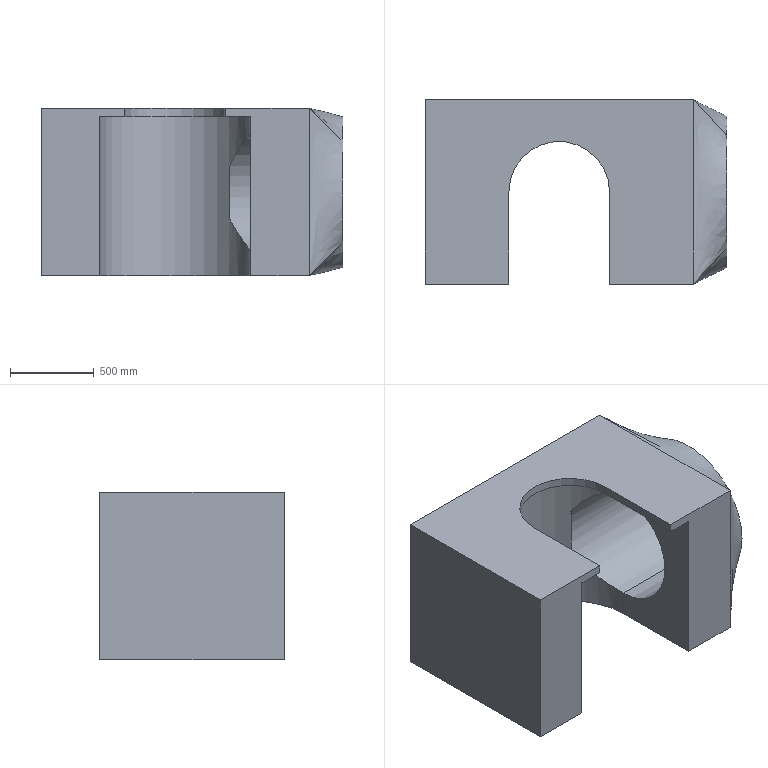Part | SolidWorks | features ICE 3, Blend 1, Extrusion 1 | 1 solid | 21 faces | box 1800 x 1100 x 1000 mm | volume 917422544 mm3 | plane 13 | cylinder 4 | spline 4 | commonest cylinder face diameters 700 x2 600 x1 900 x1
STEP:
#1=CARTESIAN_POINT('',(450.,550.,350.));
#2=VERTEX_POINT('',#1);
#3=CARTESIAN_POINT('',(450.,550.,-350.));
#4=VERTEX_POINT('',#3);
#5=CARTESIAN_POINT('',(450.,550.,0.));
#6=DIRECTION('',(1.,0.,0.));
#7=DIRECTION('',(0.,1.,0.));
#8=AXIS2_PLACEMENT_3D('',#5,#6,#7);
#9=CIRCLE('',#8,350.);
#10=EDGE_CURVE('',#2,#4,#9,.T.);
#11=ORIENTED_EDGE('',*,*,#10,.F.);
#12=CARTESIAN_POINT('',(1000.,550.,350.));
#13=VERTEX_POINT('',#12);
#14=CARTESIAN_POINT('',(324.,550.,350.));
#15=DIRECTION('',(1.,0.,0.));
#16=VECTOR('',#15,1000.);
#17=LINE('',#14,#16);
#18=EDGE_CURVE('',#2,#13,#17,.T.);
#19=ORIENTED_EDGE('',*,*,#18,.T.);
#20=CARTESIAN_POINT('',(1000.,550.,-350.));
#21=VERTEX_POINT('',#20);
#22=CARTESIAN_POINT('',(1000.,550.,0.));
#23=DIRECTION('',(1.,0.,0.));
#24=DIRECTION('',(0.,0.,-1.));
#25=AXIS2_PLACEMENT_3D('',#22,#23,#24);
#26=CIRCLE('',#25,350.);
#27=EDGE_CURVE('',#13,#21,#26,.T.);
#28=ORIENTED_EDGE('',*,*,#27,.T.);
#29=CARTESIAN_POINT('',(324.,550.,-350.));
#30=DIRECTION('',(1.,0.,0.));
#31=VECTOR('',#30,1000.);
#32=LINE('',#29,#31);
#33=EDGE_CURVE('',#4,#21,#32,.T.);
#34=ORIENTED_EDGE('',*,*,#33,.F.);
#35=EDGE_LOOP('',(#11,#19,#28,#34));
#36=FACE_OUTER_BOUND('',#35,.T.);
#37=CARTESIAN_POINT('',(324.,550.,0.));
#38=DIRECTION('',(1.,0.,0.));
#39=DIRECTION('',(0.,0.,-1.));
#40=AXIS2_PLACEMENT_3D('',#37,#38,#39);
#41=CYLINDRICAL_SURFACE('',#40,350.);
#42=ADVANCED_FACE('',(#36),#41,.F.);
#43=CARTESIAN_POINT('',(-300.,0.,500.));
#44=VERTEX_POINT('',#43);
#45=CARTESIAN_POINT('',(-300.,0.,450.));
#46=VERTEX_POINT('',#45);
#47=CARTESIAN_POINT('',(-300.,0.,500.));
#48=DIRECTION('',(0.,0.,-1.));
#49=VECTOR('',#48,1000.);
#50=LINE('',#47,#49);
#51=EDGE_CURVE('',#44,#46,#50,.T.);
#52=ORIENTED_EDGE('',*,*,#51,.F.);
#53=CARTESIAN_POINT('',(-800.,0.,500.));
#54=VERTEX_POINT('',#53);
#55=CARTESIAN_POINT('',(-800.,0.,500.));
#56=DIRECTION('',(1.,0.,0.));
#57=VECTOR('',#56,1000.);
#58=LINE('',#55,#57);
#59=EDGE_CURVE('',#54,#44,#58,.T.);
#60=ORIENTED_EDGE('',*,*,#59,.F.);
#61=CARTESIAN_POINT('',(-800.,0.,-500.));
#62=VERTEX_POINT('',#61);
#63=CARTESIAN_POINT('',(-800.,0.,500.));
#64=DIRECTION('',(0.,0.,1.));
#65=VECTOR('',#64,1000.);
#66=LINE('',#63,#65);
#67=EDGE_CURVE('',#62,#54,#66,.T.);
#68=ORIENTED_EDGE('',*,*,#67,.F.);
#69=CARTESIAN_POINT('',(-450.,0.,-500.));
#70=VERTEX_POINT('',#69);
#71=CARTESIAN_POINT('',(-800.,0.,-500.));
#72=DIRECTION('',(-1.,0.,0.));
#73=VECTOR('',#72,1000.);
#74=LINE('',#71,#73);
#75=EDGE_CURVE('',#70,#62,#74,.T.);
#76=ORIENTED_EDGE('',*,*,#75,.F.);
#77=CARTESIAN_POINT('',(-450.,0.,450.));
#78=VERTEX_POINT('',#77);
#79=CARTESIAN_POINT('',(-450.,0.,0.));
#80=DIRECTION('',(0.,0.,-1.));
#81=VECTOR('',#80,1000.);
#82=LINE('',#79,#81);
#83=EDGE_CURVE('',#78,#70,#82,.T.);
#84=ORIENTED_EDGE('',*,*,#83,.F.);
#85=CARTESIAN_POINT('',(0.,0.,450.));
#86=DIRECTION('',(1.,0.,0.));
#87=VECTOR('',#86,1000.);
#88=LINE('',#85,#87);
#89=EDGE_CURVE('',#78,#46,#88,.T.);
#90=ORIENTED_EDGE('',*,*,#89,.T.);
#91=EDGE_LOOP('',(#52,#60,#68,#76,#84,#90));
#92=FACE_OUTER_BOUND('',#91,.T.);
#93=CARTESIAN_POINT('',(0.,0.,0.));
#94=DIRECTION('',(0.,-1.,0.));
#95=DIRECTION('',(0.,0.,-1.));
#96=AXIS2_PLACEMENT_3D('',#93,#94,#95);
#97=PLANE('',#96);
#98=ADVANCED_FACE('',(#92),#97,.T.);
#99=CARTESIAN_POINT('',(-450.,550.,-500.));
#100=VERTEX_POINT('',#99);
#101=CARTESIAN_POINT('',(450.,550.,-500.));
#102=VERTEX_POINT('',#101);
#103=CARTESIAN_POINT('',(0.,550.,-500.));
#104=DIRECTION('',(0.,0.,-1.));
#105=DIRECTION('',(-1.,0.,0.));
#106=AXIS2_PLACEMENT_3D('',#103,#104,#105);
#107=CIRCLE('',#106,450.);
#108=EDGE_CURVE('',#100,#102,#107,.T.);
#109=ORIENTED_EDGE('',*,*,#108,.F.);
#110=CARTESIAN_POINT('',(-450.,550.,-500.));
#111=DIRECTION('',(0.,1.,0.));
#112=VECTOR('',#111,1000.);
#113=LINE('',#110,#112);
#114=EDGE_CURVE('',#70,#100,#113,.T.);
#115=ORIENTED_EDGE('',*,*,#114,.F.);
#116=ORIENTED_EDGE('',*,*,#75,.T.);
#117=CARTESIAN_POINT('',(-800.,1100.,-500.));
#118=VERTEX_POINT('',#117);
#119=CARTESIAN_POINT('',(-800.,1100.,-500.));
#120=DIRECTION('',(0.,-1.,0.));
#121=VECTOR('',#120,1000.);
#122=LINE('',#119,#121);
#123=EDGE_CURVE('',#118,#62,#122,.T.);
#124=ORIENTED_EDGE('',*,*,#123,.F.);
#125=CARTESIAN_POINT('',(800.,1100.,-500.));
#126=VERTEX_POINT('',#125);
#127=CARTESIAN_POINT('',(-800.,1100.,-500.));
#128=DIRECTION('',(-1.,0.,0.));
#129=VECTOR('',#128,1000.);
#130=LINE('',#127,#129);
#131=EDGE_CURVE('',#126,#118,#130,.T.);
#132=ORIENTED_EDGE('',*,*,#131,.F.);
#133=CARTESIAN_POINT('',(800.,0.,-500.));
#134=VERTEX_POINT('',#133);
#135=CARTESIAN_POINT('',(800.,1100.,-500.));
#136=DIRECTION('',(0.,-1.,0.));
#137=VECTOR('',#136,1000.);
#138=LINE('',#135,#137);
#139=EDGE_CURVE('',#126,#134,#138,.T.);
#140=ORIENTED_EDGE('',*,*,#139,.T.);
#141=CARTESIAN_POINT('',(450.,0.,-500.));
#142=VERTEX_POINT('',#141);
#143=CARTESIAN_POINT('',(-800.,0.,-500.));
#144=DIRECTION('',(-1.,0.,0.));
#145=VECTOR('',#144,1000.);
#146=LINE('',#143,#145);
#147=EDGE_CURVE('',#134,#142,#146,.T.);
#148=ORIENTED_EDGE('',*,*,#147,.T.);
#149=CARTESIAN_POINT('',(450.,550.,-500.));
#150=DIRECTION('',(0.,-1.,0.));
#151=VECTOR('',#150,1000.);
#152=LINE('',#149,#151);
#153=EDGE_CURVE('',#102,#142,#152,.T.);
#154=ORIENTED_EDGE('',*,*,#153,.F.);
#155=EDGE_LOOP('',(#109,#115,#116,#124,#132,#140,#148,#154));
#156=FACE_OUTER_BOUND('',#155,.T.);
#157=CARTESIAN_POINT('',(-800.,1100.,-500.));
#158=DIRECTION('',(0.,0.,1.));
#159=DIRECTION('',(1.,0.,0.));
#160=AXIS2_PLACEMENT_3D('',#157,#158,#159);
#161=PLANE('',#160);
#162=ADVANCED_FACE('',(#156),#161,.F.);
#163=ORIENTED_EDGE('',*,*,#67,.T.);
#164=CARTESIAN_POINT('',(-800.,1100.,500.));
#165=VERTEX_POINT('',#164);
#166=CARTESIAN_POINT('',(-800.,1100.,500.));
#167=DIRECTION('',(0.,-1.,0.));
#168=VECTOR('',#167,1000.);
#169=LINE('',#166,#168);
#170=EDGE_CURVE('',#165,#54,#169,.T.);
#171=ORIENTED_EDGE('',*,*,#170,.F.);
#172=CARTESIAN_POINT('',(-800.,1100.,500.));
#173=DIRECTION('',(0.,0.,1.));
#174=VECTOR('',#173,1000.);
#175=LINE('',#172,#174);
#176=EDGE_CURVE('',#118,#165,#175,.T.);
#177=ORIENTED_EDGE('',*,*,#176,.F.);
#178=ORIENTED_EDGE('',*,*,#123,.T.);
#179=EDGE_LOOP('',(#163,#171,#177,#178));
#180=FACE_OUTER_BOUND('',#179,.T.);
#181=CARTESIAN_POINT('',(-800.,1100.,500.));
#182=DIRECTION('',(1.,0.,0.));
#183=DIRECTION('',(0.,0.,-1.));
#184=AXIS2_PLACEMENT_3D('',#181,#182,#183);
#185=PLANE('',#184);
#186=ADVANCED_FACE('',(#180),#185,.F.);
#187=ORIENTED_EDGE('',*,*,#59,.T.);
#188=CARTESIAN_POINT('',(-300.,550.,500.));
#189=VERTEX_POINT('',#188);
#190=CARTESIAN_POINT('',(-300.,1100.,500.));
#191=DIRECTION('',(0.,1.,0.));
#192=VECTOR('',#191,1000.);
#193=LINE('',#190,#192);
#194=EDGE_CURVE('',#44,#189,#193,.T.);
#195=ORIENTED_EDGE('',*,*,#194,.T.);
#196=CARTESIAN_POINT('',(300.,550.,500.));
#197=VERTEX_POINT('',#196);
#198=CARTESIAN_POINT('',(0.,550.,500.));
#199=DIRECTION('',(0.,0.,-1.));
#200=DIRECTION('',(-1.,0.,0.));
#201=AXIS2_PLACEMENT_3D('',#198,#199,#200);
#202=CIRCLE('',#201,300.);
#203=EDGE_CURVE('',#189,#197,#202,.T.);
#204=ORIENTED_EDGE('',*,*,#203,.T.);
#205=CARTESIAN_POINT('',(300.,0.,500.));
#206=VERTEX_POINT('',#205);
#207=CARTESIAN_POINT('',(300.,1100.,500.));
#208=DIRECTION('',(0.,-1.,0.));
#209=VECTOR('',#208,1000.);
#210=LINE('',#207,#209);
#211=EDGE_CURVE('',#197,#206,#210,.T.);
#212=ORIENTED_EDGE('',*,*,#211,.T.);
#213=CARTESIAN_POINT('',(800.,0.,500.));
#214=VERTEX_POINT('',#213);
#215=CARTESIAN_POINT('',(-800.,0.,500.));
#216=DIRECTION('',(1.,0.,0.));
#217=VECTOR('',#216,1000.);
#218=LINE('',#215,#217);
#219=EDGE_CURVE('',#206,#214,#218,.T.);
#220=ORIENTED_EDGE('',*,*,#219,.T.);
#221=CARTESIAN_POINT('',(800.,1100.,500.));
#222=VERTEX_POINT('',#221);
#223=CARTESIAN_POINT('',(800.,1100.,500.));
#224=DIRECTION('',(0.,-1.,0.));
#225=VECTOR('',#224,1000.);
#226=LINE('',#223,#225);
#227=EDGE_CURVE('',#222,#214,#226,.T.);
#228=ORIENTED_EDGE('',*,*,#227,.F.);
#229=CARTESIAN_POINT('',(-800.,1100.,500.));
#230=DIRECTION('',(1.,0.,0.));
#231=VECTOR('',#230,1000.);
#232=LINE('',#229,#231);
#233=EDGE_CURVE('',#165,#222,#232,.T.);
#234=ORIENTED_EDGE('',*,*,#233,.F.);
#235=ORIENTED_EDGE('',*,*,#170,.T.);
#236=EDGE_LOOP('',(#187,#195,#204,#212,#220,#228,#234,#235));
#237=FACE_OUTER_BOUND('',#236,.T.);
#238=CARTESIAN_POINT('',(-800.,1100.,500.));
#239=DIRECTION('',(0.,0.,-1.));
#240=DIRECTION('',(-1.,0.,0.));
#241=AXIS2_PLACEMENT_3D('',#238,#239,#240);
#242=PLANE('',#241);
#243=ADVANCED_FACE('',(#237),#242,.F.);
#244=CARTESIAN_POINT('',(800.,1100.,0.));
#245=DIRECTION('',(0.,0.,-1.));
#246=VECTOR('',#245,1000.);
#247=LINE('',#244,#246);
#248=EDGE_CURVE('',#222,#126,#247,.T.);
#249=ORIENTED_EDGE('',*,*,#248,.T.);
#250=ORIENTED_EDGE('',*,*,#131,.T.);
#251=ORIENTED_EDGE('',*,*,#176,.T.);
#252=ORIENTED_EDGE('',*,*,#233,.T.);
#253=EDGE_LOOP('',(#249,#250,#251,#252));
#254=FACE_OUTER_BOUND('',#253,.T.);
#255=CARTESIAN_POINT('',(0.,1100.,0.));
#256=DIRECTION('',(0.,-1.,0.));
#257=DIRECTION('',(0.,0.,-1.));
#258=AXIS2_PLACEMENT_3D('',#255,#256,#257);
#259=PLANE('',#258);
#260=ADVANCED_FACE('',(#254),#259,.F.);
#261=CARTESIAN_POINT('',(300.,0.,450.));
#262=VERTEX_POINT('',#261);
#263=CARTESIAN_POINT('',(300.,0.,500.));
#264=DIRECTION('',(0.,0.,-1.));
#265=VECTOR('',#264,1000.);
#266=LINE('',#263,#265);
#267=EDGE_CURVE('',#206,#262,#266,.T.);
#268=ORIENTED_EDGE('',*,*,#267,.T.);
#269=CARTESIAN_POINT('',(450.,0.,450.));
#270=VERTEX_POINT('',#269);
#271=CARTESIAN_POINT('',(0.,0.,450.));
#272=DIRECTION('',(1.,0.,0.));
#273=VECTOR('',#272,1000.);
#274=LINE('',#271,#273);
#275=EDGE_CURVE('',#262,#270,#274,.T.);
#276=ORIENTED_EDGE('',*,*,#275,.T.);
#277=CARTESIAN_POINT('',(450.,0.,0.));
#278=DIRECTION('',(0.,0.,1.));
#279=VECTOR('',#278,1000.);
#280=LINE('',#277,#279);
#281=EDGE_CURVE('',#142,#270,#280,.T.);
#282=ORIENTED_EDGE('',*,*,#281,.F.);
#283=ORIENTED_EDGE('',*,*,#147,.F.);
#284=CARTESIAN_POINT('',(800.,0.,0.));
#285=DIRECTION('',(0.,0.,-1.));
#286=VECTOR('',#285,1000.);
#287=LINE('',#284,#286);
#288=EDGE_CURVE('',#214,#134,#287,.T.);
#289=ORIENTED_EDGE('',*,*,#288,.F.);
#290=ORIENTED_EDGE('',*,*,#219,.F.);
#291=EDGE_LOOP('',(#268,#276,#282,#283,#289,#290));
#292=FACE_OUTER_BOUND('',#291,.T.);
#293=CARTESIAN_POINT('',(0.,0.,0.));
#294=DIRECTION('',(0.,-1.,0.));
#295=DIRECTION('',(0.,0.,-1.));
#296=AXIS2_PLACEMENT_3D('',#293,#294,#295);
#297=PLANE('',#296);
#298=ADVANCED_FACE('',(#292),#297,.T.);
#299=CARTESIAN_POINT('',(1000.,550.,0.));
#300=DIRECTION('',(1.,0.,0.));
#301=DIRECTION('',(0.,0.,-1.));
#302=AXIS2_PLACEMENT_3D('',#299,#300,#301);
#303=CIRCLE('',#302,350.);
#304=EDGE_CURVE('',#21,#13,#303,.T.);
#305=ORIENTED_EDGE('',*,*,#304,.F.);
#306=ORIENTED_EDGE('',*,*,#27,.F.);
#307=EDGE_LOOP('',(#305,#306));
#308=FACE_BOUND('',#307,.T.);
#309=CARTESIAN_POINT('',(1000.,883.964,301.609));
#310=VERTEX_POINT('',#309);
#311=CARTESIAN_POINT('',(1000.,218.021,303.793));
#312=VERTEX_POINT('',#311);
#313=CARTESIAN_POINT('',(1000.,550.,0.));
#314=DIRECTION('',(1.,0.,0.));
#315=DIRECTION('',(0.,0.,-1.));
#316=AXIS2_PLACEMENT_3D('',#313,#314,#315);
#317=CIRCLE('',#316,450.);
#318=EDGE_CURVE('',#310,#312,#317,.T.);
#319=ORIENTED_EDGE('',*,*,#318,.T.);
#320=CARTESIAN_POINT('',(1000.,216.036,-301.609));
#321=VERTEX_POINT('',#320);
#322=CARTESIAN_POINT('',(1000.,550.,0.));
#323=DIRECTION('',(1.,0.,0.));
#324=DIRECTION('',(0.,0.,-1.));
#325=AXIS2_PLACEMENT_3D('',#322,#323,#324);
#326=CIRCLE('',#325,450.);
#327=EDGE_CURVE('',#312,#321,#326,.T.);
#328=ORIENTED_EDGE('',*,*,#327,.T.);
#329=CARTESIAN_POINT('',(1000.,881.979,-303.793));
#330=VERTEX_POINT('',#329);
#331=CARTESIAN_POINT('',(1000.,550.,0.));
#332=DIRECTION('',(1.,0.,0.));
#333=DIRECTION('',(0.,0.,-1.));
#334=AXIS2_PLACEMENT_3D('',#331,#332,#333);
#335=CIRCLE('',#334,450.);
#336=EDGE_CURVE('',#321,#330,#335,.T.);
#337=ORIENTED_EDGE('',*,*,#336,.T.);
#338=CARTESIAN_POINT('',(1000.,550.,0.));
#339=DIRECTION('',(1.,0.,0.));
#340=DIRECTION('',(0.,0.,-1.));
#341=AXIS2_PLACEMENT_3D('',#338,#339,#340);
#342=CIRCLE('',#341,450.);
#343=EDGE_CURVE('',#330,#310,#342,.T.);
#344=ORIENTED_EDGE('',*,*,#343,.T.);
#345=EDGE_LOOP('',(#319,#328,#337,#344));
#346=FACE_OUTER_BOUND('',#345,.T.);
#347=CARTESIAN_POINT('',(1000.,550.,0.));
#348=DIRECTION('',(1.,0.,0.));
#349=DIRECTION('',(0.,0.,-1.));
#350=AXIS2_PLACEMENT_3D('',#347,#348,#349);
#351=PLANE('',#350);
#352=ADVANCED_FACE('',(#308,#346),#351,.T.);
#353=ORIENTED_EDGE('',*,*,#227,.T.);
#354=CARTESIAN_POINT('',(900.,109.011,401.896));
#355=DIRECTION('',(0.5634,0.6141,-0.5527));
#356=VECTOR('',#355,1000.);
#357=LINE('',#354,#356);
#358=EDGE_CURVE('',#214,#312,#357,.T.);
#359=ORIENTED_EDGE('',*,*,#358,.T.);
#360=ORIENTED_EDGE('',*,*,#318,.F.);
#361=CARTESIAN_POINT('',(900.,991.982,400.805));
#362=DIRECTION('',(-0.5634,0.6085,0.5588));
#363=VECTOR('',#362,1000.);
#364=LINE('',#361,#363);
#365=EDGE_CURVE('',#310,#222,#364,.T.);
#366=ORIENTED_EDGE('',*,*,#365,.T.);
#367=EDGE_LOOP('',(#353,#359,#360,#366));
#368=FACE_OUTER_BOUND('',#367,.T.);
#369=CARTESIAN_POINT('',(800.,1100.,500.));
#370=CARTESIAN_POINT('',(1000.,883.964,301.609));
#371=CARTESIAN_POINT('',(800.,1077.083,500.));
#372=CARTESIAN_POINT('',(1000.,874.665,311.906));
#373=CARTESIAN_POINT('',(800.,1054.167,500.));
#374=CARTESIAN_POINT('',(1000.,864.698,321.983));
#375=CARTESIAN_POINT('',(800.,1008.333,500.));
#376=CARTESIAN_POINT('',(1000.,843.427,341.48));
#377=CARTESIAN_POINT('',(800.,985.417,500.));
#378=CARTESIAN_POINT('',(1000.,832.123,350.899));
#379=CARTESIAN_POINT('',(800.,939.583,500.));
#380=CARTESIAN_POINT('',(1000.,808.221,368.843));
#381=CARTESIAN_POINT('',(800.,916.667,500.));
#382=CARTESIAN_POINT('',(1000.,795.623,377.368));
#383=CARTESIAN_POINT('',(800.,870.833,500.));
#384=CARTESIAN_POINT('',(1000.,769.231,393.288));
#385=CARTESIAN_POINT('',(800.,847.917,500.));
#386=CARTESIAN_POINT('',(1000.,755.437,400.682));
#387=CARTESIAN_POINT('',(800.,802.083,500.));
#388=CARTESIAN_POINT('',(1000.,726.801,414.115));
#389=CARTESIAN_POINT('',(800.,779.167,500.));
#390=CARTESIAN_POINT('',(1000.,711.96,420.154));
#391=CARTESIAN_POINT('',(800.,733.333,500.));
#392=CARTESIAN_POINT('',(1000.,681.434,430.68));
#393=CARTESIAN_POINT('',(800.,710.417,500.));
#394=CARTESIAN_POINT('',(1000.,665.751,435.167));
#395=CARTESIAN_POINT('',(800.,664.583,500.));
#396=CARTESIAN_POINT('',(1000.,633.789,442.434));
#397=CARTESIAN_POINT('',(800.,641.667,500.));
#398=CARTESIAN_POINT('',(1000.,617.513,445.214));
#399=CARTESIAN_POINT('',(800.,595.833,500.));
#400=CARTESIAN_POINT('',(1000.,584.65,448.969));
#401=CARTESIAN_POINT('',(800.,572.917,500.));
#402=CARTESIAN_POINT('',(1000.,568.064,449.943));
#403=CARTESIAN_POINT('',(800.,527.083,500.));
#404=CARTESIAN_POINT('',(1000.,534.887,450.052));
#405=CARTESIAN_POINT('',(800.,504.167,500.));
#406=CARTESIAN_POINT('',(1000.,518.295,449.186));
#407=CARTESIAN_POINT('',(800.,458.333,500.));
#408=CARTESIAN_POINT('',(1000.,485.409,445.647));
#409=CARTESIAN_POINT('',(800.,435.417,500.));
#410=CARTESIAN_POINT('',(1000.,469.114,442.974));
#411=CARTESIAN_POINT('',(800.,389.583,500.));
#412=CARTESIAN_POINT('',(1000.,437.106,435.917));
#413=CARTESIAN_POINT('',(800.,366.667,500.));
#414=CARTESIAN_POINT('',(1000.,421.393,431.533));
#415=CARTESIAN_POINT('',(800.,320.833,500.));
#416=CARTESIAN_POINT('',(1000.,390.799,421.207));
#417=CARTESIAN_POINT('',(800.,297.917,500.));
#418=CARTESIAN_POINT('',(1000.,375.919,415.266));
#419=CARTESIAN_POINT('',(800.,252.083,500.));
#420=CARTESIAN_POINT('',(1000.,347.195,402.02));
#421=CARTESIAN_POINT('',(800.,229.167,500.));
#422=CARTESIAN_POINT('',(1000.,333.353,394.717));
#423=CARTESIAN_POINT('',(800.,183.333,500.));
#424=CARTESIAN_POINT('',(1000.,306.857,378.971));
#425=CARTESIAN_POINT('',(800.,160.417,500.));
#426=CARTESIAN_POINT('',(1000.,294.204,370.529));
#427=CARTESIAN_POINT('',(800.,114.583,500.));
#428=CARTESIAN_POINT('',(1000.,270.185,352.742));
#429=CARTESIAN_POINT('',(800.,91.667,500.));
#430=CARTESIAN_POINT('',(1000.,258.819,343.397));
#431=CARTESIAN_POINT('',(800.,45.833,500.));
#432=CARTESIAN_POINT('',(1000.,237.42,324.04));
#433=CARTESIAN_POINT('',(800.,22.917,500.));
#434=CARTESIAN_POINT('',(1000.,227.388,314.028));
#435=CARTESIAN_POINT('',(800.,0.,500.));
#436=CARTESIAN_POINT('',(1000.,218.021,303.793));
#437=B_SPLINE_SURFACE_WITH_KNOTS('',3,1,((#369,#370),(#371,#372),(#373,#374),(#375,#376),(#377,#378),(#379,#380),(#381,#382),(#383,#384),(#385,#386),(#387,#388),(#389,#390),(#391,#392),(#393,#394),(#395,#396),(#397,#398),(#399,#400),(#401,#402),(#403,#404),(#405,#406),(#407,#408),(#409,#410),(#411,#412),(#413,#414),(#415,#416),(#417,#418),(#419,#420),(#421,#422),(#423,#424),(#425,#426),(#427,#428),(#429,#430),(#431,#432),(#433,#434),(#435,#436)),.UNSPECIFIED.,.F.,.F.,.F.,(4,2,2,2,2,2,2,2,2,2,2,2,2,2,2,2,4),(2,2),(0.,0.0625,0.125,0.1875,0.25,0.3125,0.375,0.4375,0.5,0.5625,0.625,0.6875,0.75,0.8125,0.875,0.9375,1.),(0.,1.),.UNSPECIFIED.);
#438=ADVANCED_FACE('',(#368),#437,.T.);
#439=ORIENTED_EDGE('',*,*,#288,.T.);
#440=CARTESIAN_POINT('',(900.,108.018,-400.805));
#441=DIRECTION('',(0.5634,0.6085,0.5588));
#442=VECTOR('',#441,1000.);
#443=LINE('',#440,#442);
#444=EDGE_CURVE('',#134,#321,#443,.T.);
#445=ORIENTED_EDGE('',*,*,#444,.T.);
#446=ORIENTED_EDGE('',*,*,#327,.F.);
#447=ORIENTED_EDGE('',*,*,#358,.F.);
#448=EDGE_LOOP('',(#439,#445,#446,#447));
#449=FACE_OUTER_BOUND('',#448,.T.);
#450=CARTESIAN_POINT('',(800.,0.,500.));
#451=CARTESIAN_POINT('',(1000.,218.021,303.793));
#452=CARTESIAN_POINT('',(800.,0.,479.167));
#453=CARTESIAN_POINT('',(1000.,209.507,294.488));
#454=CARTESIAN_POINT('',(800.,0.,458.333));
#455=CARTESIAN_POINT('',(1000.,201.244,284.673));
#456=CARTESIAN_POINT('',(800.,0.,416.667));
#457=CARTESIAN_POINT('',(1000.,185.381,264.05));
#458=CARTESIAN_POINT('',(800.,0.,395.833));
#459=CARTESIAN_POINT('',(1000.,177.781,253.242));
#460=CARTESIAN_POINT('',(800.,0.,354.167));
#461=CARTESIAN_POINT('',(1000.,163.399,230.691));
#462=CARTESIAN_POINT('',(800.,0.,333.333));
#463=CARTESIAN_POINT('',(1000.,156.618,218.948));
#464=CARTESIAN_POINT('',(800.,0.,291.667));
#465=CARTESIAN_POINT('',(1000.,144.029,194.616));
#466=CARTESIAN_POINT('',(800.,0.,270.833));
#467=CARTESIAN_POINT('',(1000.,138.221,182.026));
#468=CARTESIAN_POINT('',(800.,0.,229.167));
#469=CARTESIAN_POINT('',(1000.,127.719,156.123));
#470=CARTESIAN_POINT('',(800.,0.,208.333));
#471=CARTESIAN_POINT('',(1000.,123.026,142.809));
#472=CARTESIAN_POINT('',(800.,0.,166.667));
#473=CARTESIAN_POINT('',(1000.,114.872,115.607));
#474=CARTESIAN_POINT('',(800.,0.,145.833));
#475=CARTESIAN_POINT('',(1000.,111.412,101.718));
#476=CARTESIAN_POINT('',(800.,0.,104.167));
#477=CARTESIAN_POINT('',(1000.,105.818,73.541));
#478=CARTESIAN_POINT('',(800.,0.,83.333));
#479=CARTESIAN_POINT('',(1000.,103.684,59.252));
#480=CARTESIAN_POINT('',(800.,0.,41.667));
#481=CARTESIAN_POINT('',(1000.,100.8,30.468));
#482=CARTESIAN_POINT('',(800.,0.,20.833));
#483=CARTESIAN_POINT('',(1000.,100.05,15.973));
#484=CARTESIAN_POINT('',(800.,0.,-20.833));
#485=CARTESIAN_POINT('',(1000.,99.955,-13.022));
#486=CARTESIAN_POINT('',(800.,0.,-41.667));
#487=CARTESIAN_POINT('',(1000.,100.61,-27.522));
#488=CARTESIAN_POINT('',(800.,0.,-83.333));
#489=CARTESIAN_POINT('',(1000.,103.305,-56.324));
#490=CARTESIAN_POINT('',(800.,0.,-104.167));
#491=CARTESIAN_POINT('',(1000.,105.345,-70.626));
#492=CARTESIAN_POINT('',(800.,0.,-145.833));
#493=CARTESIAN_POINT('',(1000.,110.754,-98.839));
#494=CARTESIAN_POINT('',(800.,0.,-166.667));
#495=CARTESIAN_POINT('',(1000.,114.123,-112.75));
#496=CARTESIAN_POINT('',(800.,0.,-208.333));
#497=CARTESIAN_POINT('',(1000.,122.098,-140.006));
#498=CARTESIAN_POINT('',(800.,0.,-229.167));
#499=CARTESIAN_POINT('',(1000.,126.705,-153.351));
#500=CARTESIAN_POINT('',(800.,0.,-270.833));
#501=CARTESIAN_POINT('',(1000.,137.036,-179.322));
#502=CARTESIAN_POINT('',(800.,0.,-291.667));
#503=CARTESIAN_POINT('',(1000.,142.761,-191.949));
#504=CARTESIAN_POINT('',(800.,0.,-333.333));
#505=CARTESIAN_POINT('',(1000.,155.191,-216.363));
#506=CARTESIAN_POINT('',(800.,0.,-354.167));
#507=CARTESIAN_POINT('',(1000.,161.894,-228.151));
#508=CARTESIAN_POINT('',(800.,0.,-395.833));
#509=CARTESIAN_POINT('',(1000.,176.128,-250.796));
#510=CARTESIAN_POINT('',(800.,0.,-416.667));
#511=CARTESIAN_POINT('',(1000.,183.658,-261.653));
#512=CARTESIAN_POINT('',(800.,0.,-458.333));
#513=CARTESIAN_POINT('',(1000.,199.385,-282.38));
#514=CARTESIAN_POINT('',(800.,0.,-479.167));
#515=CARTESIAN_POINT('',(1000.,207.583,-292.249));
#516=CARTESIAN_POINT('',(800.,0.,-500.));
#517=CARTESIAN_POINT('',(1000.,216.036,-301.609));
#518=B_SPLINE_SURFACE_WITH_KNOTS('',3,1,((#450,#451),(#452,#453),(#454,#455),(#456,#457),(#458,#459),(#460,#461),(#462,#463),(#464,#465),(#466,#467),(#468,#469),(#470,#471),(#472,#473),(#474,#475),(#476,#477),(#478,#479),(#480,#481),(#482,#483),(#484,#485),(#486,#487),(#488,#489),(#490,#491),(#492,#493),(#494,#495),(#496,#497),(#498,#499),(#500,#501),(#502,#503),(#504,#505),(#506,#507),(#508,#509),(#510,#511),(#512,#513),(#514,#515),(#516,#517)),.UNSPECIFIED.,.F.,.F.,.F.,(4,2,2,2,2,2,2,2,2,2,2,2,2,2,2,2,4),(2,2),(0.,0.0625,0.125,0.1875,0.25,0.3125,0.375,0.4375,0.5,0.5625,0.625,0.6875,0.75,0.8125,0.875,0.9375,1.),(0.,1.),.UNSPECIFIED.);
#519=ADVANCED_FACE('',(#449),#518,.T.);
#520=ORIENTED_EDGE('',*,*,#248,.F.);
#521=ORIENTED_EDGE('',*,*,#365,.F.);
#522=ORIENTED_EDGE('',*,*,#343,.F.);
#523=CARTESIAN_POINT('',(900.,990.989,-401.896));
#524=DIRECTION('',(0.5634,-0.6141,0.5527));
#525=VECTOR('',#524,1000.);
#526=LINE('',#523,#525);
#527=EDGE_CURVE('',#126,#330,#526,.T.);
#528=ORIENTED_EDGE('',*,*,#527,.F.);
#529=EDGE_LOOP('',(#520,#521,#522,#528));
#530=FACE_OUTER_BOUND('',#529,.T.);
#531=CARTESIAN_POINT('',(800.,1100.,-500.));
#532=CARTESIAN_POINT('',(1000.,881.979,-303.793));
#533=CARTESIAN_POINT('',(800.,1100.,-479.167));
#534=CARTESIAN_POINT('',(1000.,890.493,-294.488));
#535=CARTESIAN_POINT('',(800.,1100.,-458.333));
#536=CARTESIAN_POINT('',(1000.,898.756,-284.673));
#537=CARTESIAN_POINT('',(800.,1100.,-416.667));
#538=CARTESIAN_POINT('',(1000.,914.619,-264.05));
#539=CARTESIAN_POINT('',(800.,1100.,-395.833));
#540=CARTESIAN_POINT('',(1000.,922.219,-253.242));
#541=CARTESIAN_POINT('',(800.,1100.,-354.167));
#542=CARTESIAN_POINT('',(1000.,936.601,-230.691));
#543=CARTESIAN_POINT('',(800.,1100.,-333.333));
#544=CARTESIAN_POINT('',(1000.,943.382,-218.948));
#545=CARTESIAN_POINT('',(800.,1100.,-291.667));
#546=CARTESIAN_POINT('',(1000.,955.971,-194.616));
#547=CARTESIAN_POINT('',(800.,1100.,-270.833));
#548=CARTESIAN_POINT('',(1000.,961.779,-182.026));
#549=CARTESIAN_POINT('',(800.,1100.,-229.167));
#550=CARTESIAN_POINT('',(1000.,972.281,-156.123));
#551=CARTESIAN_POINT('',(800.,1100.,-208.333));
#552=CARTESIAN_POINT('',(1000.,976.974,-142.809));
#553=CARTESIAN_POINT('',(800.,1100.,-166.667));
#554=CARTESIAN_POINT('',(1000.,985.128,-115.607));
#555=CARTESIAN_POINT('',(800.,1100.,-145.833));
#556=CARTESIAN_POINT('',(1000.,988.588,-101.718));
#557=CARTESIAN_POINT('',(800.,1100.,-104.167));
#558=CARTESIAN_POINT('',(1000.,994.182,-73.541));
#559=CARTESIAN_POINT('',(800.,1100.,-83.333));
#560=CARTESIAN_POINT('',(1000.,996.316,-59.252));
#561=CARTESIAN_POINT('',(800.,1100.,-41.667));
#562=CARTESIAN_POINT('',(1000.,999.2,-30.468));
#563=CARTESIAN_POINT('',(800.,1100.,-20.833));
#564=CARTESIAN_POINT('',(1000.,999.95,-15.973));
#565=CARTESIAN_POINT('',(800.,1100.,20.833));
#566=CARTESIAN_POINT('',(1000.,1000.045,13.022));
#567=CARTESIAN_POINT('',(800.,1100.,41.667));
#568=CARTESIAN_POINT('',(1000.,999.39,27.522));
#569=CARTESIAN_POINT('',(800.,1100.,83.333));
#570=CARTESIAN_POINT('',(1000.,996.695,56.324));
#571=CARTESIAN_POINT('',(800.,1100.,104.167));
#572=CARTESIAN_POINT('',(1000.,994.655,70.626));
#573=CARTESIAN_POINT('',(800.,1100.,145.833));
#574=CARTESIAN_POINT('',(1000.,989.246,98.839));
#575=CARTESIAN_POINT('',(800.,1100.,166.667));
#576=CARTESIAN_POINT('',(1000.,985.877,112.75));
#577=CARTESIAN_POINT('',(800.,1100.,208.333));
#578=CARTESIAN_POINT('',(1000.,977.902,140.006));
#579=CARTESIAN_POINT('',(800.,1100.,229.167));
#580=CARTESIAN_POINT('',(1000.,973.295,153.351));
#581=CARTESIAN_POINT('',(800.,1100.,270.833));
#582=CARTESIAN_POINT('',(1000.,962.964,179.322));
#583=CARTESIAN_POINT('',(800.,1100.,291.667));
#584=CARTESIAN_POINT('',(1000.,957.239,191.949));
#585=CARTESIAN_POINT('',(800.,1100.,333.333));
#586=CARTESIAN_POINT('',(1000.,944.809,216.363));
#587=CARTESIAN_POINT('',(800.,1100.,354.167));
#588=CARTESIAN_POINT('',(1000.,938.106,228.151));
#589=CARTESIAN_POINT('',(800.,1100.,395.833));
#590=CARTESIAN_POINT('',(1000.,923.872,250.796));
#591=CARTESIAN_POINT('',(800.,1100.,416.667));
#592=CARTESIAN_POINT('',(1000.,916.342,261.653));
#593=CARTESIAN_POINT('',(800.,1100.,458.333));
#594=CARTESIAN_POINT('',(1000.,900.615,282.38));
#595=CARTESIAN_POINT('',(800.,1100.,479.167));
#596=CARTESIAN_POINT('',(1000.,892.417,292.249));
#597=CARTESIAN_POINT('',(800.,1100.,500.));
#598=CARTESIAN_POINT('',(1000.,883.964,301.609));
#599=B_SPLINE_SURFACE_WITH_KNOTS('',3,1,((#531,#532),(#533,#534),(#535,#536),(#537,#538),(#539,#540),(#541,#542),(#543,#544),(#545,#546),(#547,#548),(#549,#550),(#551,#552),(#553,#554),(#555,#556),(#557,#558),(#559,#560),(#561,#562),(#563,#564),(#565,#566),(#567,#568),(#569,#570),(#571,#572),(#573,#574),(#575,#576),(#577,#578),(#579,#580),(#581,#582),(#583,#584),(#585,#586),(#587,#588),(#589,#590),(#591,#592),(#593,#594),(#595,#596),(#597,#598)),.UNSPECIFIED.,.F.,.F.,.F.,(4,2,2,2,2,2,2,2,2,2,2,2,2,2,2,2,4),(2,2),(0.,0.0625,0.125,0.1875,0.25,0.3125,0.375,0.4375,0.5,0.5625,0.625,0.6875,0.75,0.8125,0.875,0.9375,1.),(0.,1.),.UNSPECIFIED.);
#600=ADVANCED_FACE('',(#530),#599,.T.);
#601=ORIENTED_EDGE('',*,*,#139,.F.);
#602=ORIENTED_EDGE('',*,*,#527,.T.);
#603=ORIENTED_EDGE('',*,*,#336,.F.);
#604=ORIENTED_EDGE('',*,*,#444,.F.);
#605=EDGE_LOOP('',(#601,#602,#603,#604));
#606=FACE_OUTER_BOUND('',#605,.T.);
#607=CARTESIAN_POINT('',(800.,0.,-500.));
#608=CARTESIAN_POINT('',(1000.,216.036,-301.609));
#609=CARTESIAN_POINT('',(800.,22.917,-500.));
#610=CARTESIAN_POINT('',(1000.,225.335,-311.906));
#611=CARTESIAN_POINT('',(800.,45.833,-500.));
#612=CARTESIAN_POINT('',(1000.,235.302,-321.983));
#613=CARTESIAN_POINT('',(800.,91.667,-500.));
#614=CARTESIAN_POINT('',(1000.,256.573,-341.48));
#615=CARTESIAN_POINT('',(800.,114.583,-500.));
#616=CARTESIAN_POINT('',(1000.,267.877,-350.899));
#617=CARTESIAN_POINT('',(800.,160.417,-500.));
#618=CARTESIAN_POINT('',(1000.,291.779,-368.843));
#619=CARTESIAN_POINT('',(800.,183.333,-500.));
#620=CARTESIAN_POINT('',(1000.,304.377,-377.368));
#621=CARTESIAN_POINT('',(800.,229.167,-500.));
#622=CARTESIAN_POINT('',(1000.,330.769,-393.288));
#623=CARTESIAN_POINT('',(800.,252.083,-500.));
#624=CARTESIAN_POINT('',(1000.,344.563,-400.682));
#625=CARTESIAN_POINT('',(800.,297.917,-500.));
#626=CARTESIAN_POINT('',(1000.,373.199,-414.115));
#627=CARTESIAN_POINT('',(800.,320.833,-500.));
#628=CARTESIAN_POINT('',(1000.,388.04,-420.154));
#629=CARTESIAN_POINT('',(800.,366.667,-500.));
#630=CARTESIAN_POINT('',(1000.,418.566,-430.68));
#631=CARTESIAN_POINT('',(800.,389.583,-500.));
#632=CARTESIAN_POINT('',(1000.,434.249,-435.167));
#633=CARTESIAN_POINT('',(800.,435.417,-500.));
#634=CARTESIAN_POINT('',(1000.,466.211,-442.434));
#635=CARTESIAN_POINT('',(800.,458.333,-500.));
#636=CARTESIAN_POINT('',(1000.,482.487,-445.214));
#637=CARTESIAN_POINT('',(800.,504.167,-500.));
#638=CARTESIAN_POINT('',(1000.,515.35,-448.969));
#639=CARTESIAN_POINT('',(800.,527.083,-500.));
#640=CARTESIAN_POINT('',(1000.,531.936,-449.943));
#641=CARTESIAN_POINT('',(800.,572.917,-500.));
#642=CARTESIAN_POINT('',(1000.,565.113,-450.052));
#643=CARTESIAN_POINT('',(800.,595.833,-500.));
#644=CARTESIAN_POINT('',(1000.,581.705,-449.186));
#645=CARTESIAN_POINT('',(800.,641.667,-500.));
#646=CARTESIAN_POINT('',(1000.,614.591,-445.647));
#647=CARTESIAN_POINT('',(800.,664.583,-500.));
#648=CARTESIAN_POINT('',(1000.,630.886,-442.974));
#649=CARTESIAN_POINT('',(800.,710.417,-500.));
#650=CARTESIAN_POINT('',(1000.,662.894,-435.917));
#651=CARTESIAN_POINT('',(800.,733.333,-500.));
#652=CARTESIAN_POINT('',(1000.,678.607,-431.533));
#653=CARTESIAN_POINT('',(800.,779.167,-500.));
#654=CARTESIAN_POINT('',(1000.,709.201,-421.207));
#655=CARTESIAN_POINT('',(800.,802.083,-500.));
#656=CARTESIAN_POINT('',(1000.,724.081,-415.266));
#657=CARTESIAN_POINT('',(800.,847.917,-500.));
#658=CARTESIAN_POINT('',(1000.,752.805,-402.02));
#659=CARTESIAN_POINT('',(800.,870.833,-500.));
#660=CARTESIAN_POINT('',(1000.,766.647,-394.717));
#661=CARTESIAN_POINT('',(800.,916.667,-500.));
#662=CARTESIAN_POINT('',(1000.,793.143,-378.971));
#663=CARTESIAN_POINT('',(800.,939.583,-500.));
#664=CARTESIAN_POINT('',(1000.,805.796,-370.529));
#665=CARTESIAN_POINT('',(800.,985.417,-500.));
#666=CARTESIAN_POINT('',(1000.,829.815,-352.742));
#667=CARTESIAN_POINT('',(800.,1008.333,-500.));
#668=CARTESIAN_POINT('',(1000.,841.181,-343.397));
#669=CARTESIAN_POINT('',(800.,1054.167,-500.));
#670=CARTESIAN_POINT('',(1000.,862.58,-324.04));
#671=CARTESIAN_POINT('',(800.,1077.083,-500.));
#672=CARTESIAN_POINT('',(1000.,872.612,-314.028));
#673=CARTESIAN_POINT('',(800.,1100.,-500.));
#674=CARTESIAN_POINT('',(1000.,881.979,-303.793));
#675=B_SPLINE_SURFACE_WITH_KNOTS('',3,1,((#607,#608),(#609,#610),(#611,#612),(#613,#614),(#615,#616),(#617,#618),(#619,#620),(#621,#622),(#623,#624),(#625,#626),(#627,#628),(#629,#630),(#631,#632),(#633,#634),(#635,#636),(#637,#638),(#639,#640),(#641,#642),(#643,#644),(#645,#646),(#647,#648),(#649,#650),(#651,#652),(#653,#654),(#655,#656),(#657,#658),(#659,#660),(#661,#662),(#663,#664),(#665,#666),(#667,#668),(#669,#670),(#671,#672),(#673,#674)),.UNSPECIFIED.,.F.,.F.,.F.,(4,2,2,2,2,2,2,2,2,2,2,2,2,2,2,2,4),(2,2),(0.,0.0625,0.125,0.1875,0.25,0.3125,0.375,0.4375,0.5,0.5625,0.625,0.6875,0.75,0.8125,0.875,0.9375,1.),(0.,1.),.UNSPECIFIED.);
#676=ADVANCED_FACE('',(#606),#675,.T.);
#677=CARTESIAN_POINT('',(450.,550.,450.));
#678=DIRECTION('',(0.,0.,-1.));
#679=VECTOR('',#678,1000.);
#680=LINE('',#677,#679);
#681=EDGE_CURVE('',#4,#102,#680,.T.);
#682=ORIENTED_EDGE('',*,*,#681,.F.);
#683=CARTESIAN_POINT('',(324.,862.288,-158.038));
#684=VERTEX_POINT('',#683);
#685=CARTESIAN_POINT('',(450.,550.,-350.));
#686=CARTESIAN_POINT('',(450.,558.615,-350.));
#687=CARTESIAN_POINT('',(449.753,567.156,-349.682));
#688=CARTESIAN_POINT('',(448.787,584.096,-348.439));
#689=CARTESIAN_POINT('',(448.067,592.496,-347.513));
#690=CARTESIAN_POINT('',(446.173,609.158,-345.067));
#691=CARTESIAN_POINT('',(444.998,617.42,-343.548));
#692=CARTESIAN_POINT('',(442.903,629.713,-340.828));
#693=CARTESIAN_POINT('',(442.149,633.793,-339.848));
#694=CARTESIAN_POINT('',(440.531,641.92,-337.74));
#695=CARTESIAN_POINT('',(439.667,645.969,-336.612));
#696=CARTESIAN_POINT('',(436.913,658.053,-333.009));
#697=CARTESIAN_POINT('',(434.886,665.926,-330.347));
#698=CARTESIAN_POINT('',(430.484,681.33,-324.531));
#699=CARTESIAN_POINT('',(428.11,688.862,-321.377));
#700=CARTESIAN_POINT('',(423.044,703.604,-314.597));
#701=CARTESIAN_POINT('',(420.353,710.814,-310.972));
#702=CARTESIAN_POINT('',(416.097,721.398,-305.186));
#703=CARTESIAN_POINT('',(414.643,724.888,-303.2));
#704=CARTESIAN_POINT('',(412.408,730.065,-300.134));
#705=CARTESIAN_POINT('',(411.654,731.781,-299.098));
#706=CARTESIAN_POINT('',(410.13,735.194,-296.997));
#707=CARTESIAN_POINT('',(409.359,736.893,-295.931));
#708=CARTESIAN_POINT('',(405.468,745.322,-290.54));
#709=CARTESIAN_POINT('',(402.255,751.846,-286.042));
#710=CARTESIAN_POINT('',(395.658,764.489,-276.688));
#711=CARTESIAN_POINT('',(392.275,770.608,-271.832));
#712=CARTESIAN_POINT('',(385.369,782.461,-261.768));
#713=CARTESIAN_POINT('',(381.846,788.195,-256.56));
#714=CARTESIAN_POINT('',(374.693,799.296,-245.787));
#715=CARTESIAN_POINT('',(371.063,804.662,-240.223));
#716=CARTESIAN_POINT('',(365.56,812.442,-231.601));
#717=CARTESIAN_POINT('',(363.715,814.993,-228.678));
#718=CARTESIAN_POINT('',(360.026,819.983,-222.765));
#719=CARTESIAN_POINT('',(358.182,822.424,-219.773));
#720=CARTESIAN_POINT('',(352.655,829.591,-210.686));
#721=CARTESIAN_POINT('',(348.978,834.159,-204.482));
#722=CARTESIAN_POINT('',(341.684,842.89,-191.768));
#723=CARTESIAN_POINT('',(338.066,847.052,-185.258));
#724=CARTESIAN_POINT('',(330.938,854.973,-171.906));
#725=CARTESIAN_POINT('',(327.427,858.733,-165.064));
#726=CARTESIAN_POINT('',(324.,862.288,-158.038));
#727=B_SPLINE_CURVE_WITH_KNOTS('',3,(#685,#686,#687,#688,#689,#690,#691,#692,#693,#694,#695,#696,#697,#698,#699,#700,#701,#702,#703,#704,#705,#706,#707,#708,#709,#710,#711,#712,#713,#714,#715,#716,#717,#718,#719,#720,#721,#722,#723,#724,#725,#726),.UNSPECIFIED.,.F.,.F.,(4,2,2,2,2,2,2,2,2,2,2,2,2,2,2,2,2,2,2,2,4),(0.,0.02542,0.05084,0.07626,0.08897,0.1017,0.1271,0.1525,0.1779,0.1907,0.197,0.2034,0.2288,0.2542,0.2796,0.305,0.3178,0.3305,0.3559,0.3813,0.4067),.UNSPECIFIED.);
#728=EDGE_CURVE('',#4,#684,#727,.T.);
#729=ORIENTED_EDGE('',*,*,#728,.T.);
#730=CARTESIAN_POINT('',(324.,862.288,158.038));
#731=VERTEX_POINT('',#730);
#732=CARTESIAN_POINT('',(324.,862.288,450.));
#733=DIRECTION('',(0.,0.,-1.));
#734=VECTOR('',#733,1000.);
#735=LINE('',#732,#734);
#736=EDGE_CURVE('',#731,#684,#735,.T.);
#737=ORIENTED_EDGE('',*,*,#736,.F.);
#738=CARTESIAN_POINT('',(324.,862.288,158.038));
#739=CARTESIAN_POINT('',(327.434,858.725,165.079));
#740=CARTESIAN_POINT('',(330.946,854.964,171.922));
#741=CARTESIAN_POINT('',(338.066,847.052,185.257));
#742=CARTESIAN_POINT('',(341.673,842.902,191.748));
#743=CARTESIAN_POINT('',(348.934,834.213,204.407));
#744=CARTESIAN_POINT('',(352.589,829.673,210.574));
#745=CARTESIAN_POINT('',(359.902,820.197,222.603));
#746=CARTESIAN_POINT('',(363.561,815.26,228.465));
#747=CARTESIAN_POINT('',(370.849,804.973,239.892));
#748=CARTESIAN_POINT('',(374.477,799.622,245.457));
#749=CARTESIAN_POINT('',(379.869,791.268,253.584));
#750=CARTESIAN_POINT('',(381.659,788.429,256.256));
#751=CARTESIAN_POINT('',(385.217,782.636,261.526));
#752=CARTESIAN_POINT('',(386.976,779.699,264.11));
#753=CARTESIAN_POINT('',(392.187,770.764,271.706));
#754=CARTESIAN_POINT('',(395.573,764.644,276.567));
#755=CARTESIAN_POINT('',(402.143,752.069,285.884));
#756=CARTESIAN_POINT('',(405.326,745.613,290.34));
#757=CARTESIAN_POINT('',(411.462,732.352,298.847));
#758=CARTESIAN_POINT('',(414.415,725.547,302.897));
#759=CARTESIAN_POINT('',(420.062,711.568,310.579));
#760=CARTESIAN_POINT('',(422.757,704.394,314.211));
#761=CARTESIAN_POINT('',(427.854,689.65,321.036));
#762=CARTESIAN_POINT('',(430.256,682.08,324.229));
#763=CARTESIAN_POINT('',(433.054,672.347,327.926));
#764=CARTESIAN_POINT('',(433.602,670.389,328.65));
#765=CARTESIAN_POINT('',(434.672,666.464,330.061));
#766=CARTESIAN_POINT('',(435.195,664.496,330.749));
#767=CARTESIAN_POINT('',(436.725,658.573,332.76));
#768=CARTESIAN_POINT('',(437.694,654.599,334.031));
#769=CARTESIAN_POINT('',(440.445,642.604,337.63));
#770=CARTESIAN_POINT('',(442.072,634.508,339.748));
#771=CARTESIAN_POINT('',(444.893,618.111,343.412));
#772=CARTESIAN_POINT('',(446.088,609.81,344.956));
#773=CARTESIAN_POINT('',(447.538,597.2,346.829));
#774=CARTESIAN_POINT('',(447.964,592.97,347.379));
#775=CARTESIAN_POINT('',(448.516,586.583,348.089));
#776=CARTESIAN_POINT('',(448.685,584.448,348.307));
#777=CARTESIAN_POINT('',(448.993,580.163,348.704));
#778=CARTESIAN_POINT('',(449.132,578.013,348.884));
#779=CARTESIAN_POINT('',(449.751,567.264,349.68));
#780=CARTESIAN_POINT('',(450.,558.643,350.));
#781=CARTESIAN_POINT('',(450.,550.,350.));
#782=B_SPLINE_CURVE_WITH_KNOTS('',3,(#738,#739,#740,#741,#742,#743,#744,#745,#746,#747,#748,#749,#750,#751,#752,#753,#754,#755,#756,#757,#758,#759,#760,#761,#762,#763,#764,#765,#766,#767,#768,#769,#770,#771,#772,#773,#774,#775,#776,#777,#778,#779,#780,#781),.UNSPECIFIED.,.F.,.F.,(4,2,2,2,2,2,2,2,2,2,2,2,2,2,2,2,2,2,2,2,2,4),(0.,0.02545,0.0509,0.07636,0.1018,0.1273,0.14,0.1527,0.1782,0.2036,0.2291,0.2545,0.28,0.2863,0.2927,0.3054,0.3309,0.3563,0.369,0.3754,0.3818,0.4072),.UNSPECIFIED.);
#783=EDGE_CURVE('',#731,#2,#782,.T.);
#784=ORIENTED_EDGE('',*,*,#783,.T.);
#785=CARTESIAN_POINT('',(450.,550.,450.));
#786=VERTEX_POINT('',#785);
#787=CARTESIAN_POINT('',(450.,550.,450.));
#788=DIRECTION('',(0.,0.,-1.));
#789=VECTOR('',#788,1000.);
#790=LINE('',#787,#789);
#791=EDGE_CURVE('',#786,#2,#790,.T.);
#792=ORIENTED_EDGE('',*,*,#791,.F.);
#793=CARTESIAN_POINT('',(-450.,550.,450.));
#794=VERTEX_POINT('',#793);
#795=CARTESIAN_POINT('',(0.,550.,450.));
#796=DIRECTION('',(0.,0.,-1.));
#797=DIRECTION('',(-1.,0.,0.));
#798=AXIS2_PLACEMENT_3D('',#795,#796,#797);
#799=CIRCLE('',#798,450.);
#800=EDGE_CURVE('',#794,#786,#799,.T.);
#801=ORIENTED_EDGE('',*,*,#800,.F.);
#802=CARTESIAN_POINT('',(-450.,550.,450.));
#803=DIRECTION('',(0.,0.,-1.));
#804=VECTOR('',#803,1000.);
#805=LINE('',#802,#804);
#806=EDGE_CURVE('',#794,#100,#805,.T.);
#807=ORIENTED_EDGE('',*,*,#806,.T.);
#808=ORIENTED_EDGE('',*,*,#108,.T.);
#809=EDGE_LOOP('',(#682,#729,#737,#784,#792,#801,#807,#808));
#810=FACE_OUTER_BOUND('',#809,.T.);
#811=CARTESIAN_POINT('',(0.,550.,450.));
#812=DIRECTION('',(0.,0.,-1.));
#813=DIRECTION('',(-1.,0.,0.));
#814=AXIS2_PLACEMENT_3D('',#811,#812,#813);
#815=CYLINDRICAL_SURFACE('',#814,450.);
#816=ADVANCED_FACE('',(#810),#815,.F.);
#817=ORIENTED_EDGE('',*,*,#83,.T.);
#818=ORIENTED_EDGE('',*,*,#114,.T.);
#819=ORIENTED_EDGE('',*,*,#806,.F.);
#820=CARTESIAN_POINT('',(-450.,550.,450.));
#821=DIRECTION('',(0.,1.,0.));
#822=VECTOR('',#821,1000.);
#823=LINE('',#820,#822);
#824=EDGE_CURVE('',#78,#794,#823,.T.);
#825=ORIENTED_EDGE('',*,*,#824,.F.);
#826=EDGE_LOOP('',(#817,#818,#819,#825));
#827=FACE_OUTER_BOUND('',#826,.T.);
#828=CARTESIAN_POINT('',(-450.,550.,450.));
#829=DIRECTION('',(-1.,0.,0.));
#830=DIRECTION('',(0.,0.,1.));
#831=AXIS2_PLACEMENT_3D('',#828,#829,#830);
#832=PLANE('',#831);
#833=ADVANCED_FACE('',(#827),#832,.F.);
#834=ORIENTED_EDGE('',*,*,#791,.T.);
#835=ORIENTED_EDGE('',*,*,#10,.T.);
#836=ORIENTED_EDGE('',*,*,#681,.T.);
#837=ORIENTED_EDGE('',*,*,#153,.T.);
#838=ORIENTED_EDGE('',*,*,#281,.T.);
#839=CARTESIAN_POINT('',(450.,550.,450.));
#840=DIRECTION('',(0.,-1.,0.));
#841=VECTOR('',#840,1000.);
#842=LINE('',#839,#841);
#843=EDGE_CURVE('',#786,#270,#842,.T.);
#844=ORIENTED_EDGE('',*,*,#843,.F.);
#845=EDGE_LOOP('',(#834,#835,#836,#837,#838,#844));
#846=FACE_OUTER_BOUND('',#845,.T.);
#847=CARTESIAN_POINT('',(450.,550.,450.));
#848=DIRECTION('',(1.,0.,0.));
#849=DIRECTION('',(0.,1.,0.));
#850=AXIS2_PLACEMENT_3D('',#847,#848,#849);
#851=PLANE('',#850);
#852=ADVANCED_FACE('',(#846),#851,.F.);
#853=CARTESIAN_POINT('',(-300.,550.,450.));
#854=VERTEX_POINT('',#853);
#855=CARTESIAN_POINT('',(-300.,550.,450.));
#856=DIRECTION('',(0.,1.,0.));
#857=VECTOR('',#856,1000.);
#858=LINE('',#855,#857);
#859=EDGE_CURVE('',#46,#854,#858,.T.);
#860=ORIENTED_EDGE('',*,*,#859,.F.);
#861=ORIENTED_EDGE('',*,*,#89,.F.);
#862=ORIENTED_EDGE('',*,*,#824,.T.);
#863=ORIENTED_EDGE('',*,*,#800,.T.);
#864=ORIENTED_EDGE('',*,*,#843,.T.);
#865=ORIENTED_EDGE('',*,*,#275,.F.);
#866=CARTESIAN_POINT('',(300.,550.,450.));
#867=VERTEX_POINT('',#866);
#868=CARTESIAN_POINT('',(300.,550.,450.));
#869=DIRECTION('',(0.,-1.,0.));
#870=VECTOR('',#869,1000.);
#871=LINE('',#868,#870);
#872=EDGE_CURVE('',#867,#262,#871,.T.);
#873=ORIENTED_EDGE('',*,*,#872,.F.);
#874=CARTESIAN_POINT('',(0.,550.,450.));
#875=DIRECTION('',(0.,0.,-1.));
#876=DIRECTION('',(-1.,0.,0.));
#877=AXIS2_PLACEMENT_3D('',#874,#875,#876);
#878=CIRCLE('',#877,300.);
#879=EDGE_CURVE('',#854,#867,#878,.T.);
#880=ORIENTED_EDGE('',*,*,#879,.F.);
#881=EDGE_LOOP('',(#860,#861,#862,#863,#864,#865,#873,#880));
#882=FACE_OUTER_BOUND('',#881,.T.);
#883=CARTESIAN_POINT('',(0.,550.,450.));
#884=DIRECTION('',(0.,0.,-1.));
#885=DIRECTION('',(-1.,0.,0.));
#886=AXIS2_PLACEMENT_3D('',#883,#884,#885);
#887=PLANE('',#886);
#888=ADVANCED_FACE('',(#882),#887,.T.);
#889=CARTESIAN_POINT('',(-300.,550.,500.));
#890=DIRECTION('',(0.,0.,-1.));
#891=VECTOR('',#890,1000.);
#892=LINE('',#889,#891);
#893=EDGE_CURVE('',#189,#854,#892,.T.);
#894=ORIENTED_EDGE('',*,*,#893,.T.);
#895=ORIENTED_EDGE('',*,*,#879,.T.);
#896=CARTESIAN_POINT('',(300.,550.,500.));
#897=DIRECTION('',(0.,0.,-1.));
#898=VECTOR('',#897,1000.);
#899=LINE('',#896,#898);
#900=EDGE_CURVE('',#197,#867,#899,.T.);
#901=ORIENTED_EDGE('',*,*,#900,.F.);
#902=ORIENTED_EDGE('',*,*,#203,.F.);
#903=EDGE_LOOP('',(#894,#895,#901,#902));
#904=FACE_OUTER_BOUND('',#903,.T.);
#905=CARTESIAN_POINT('',(0.,550.,500.));
#906=DIRECTION('',(0.,0.,-1.));
#907=DIRECTION('',(-1.,0.,0.));
#908=AXIS2_PLACEMENT_3D('',#905,#906,#907);
#909=CYLINDRICAL_SURFACE('',#908,300.);
#910=ADVANCED_FACE('',(#904),#909,.F.);
#911=ORIENTED_EDGE('',*,*,#51,.T.);
#912=ORIENTED_EDGE('',*,*,#859,.T.);
#913=ORIENTED_EDGE('',*,*,#893,.F.);
#914=ORIENTED_EDGE('',*,*,#194,.F.);
#915=EDGE_LOOP('',(#911,#912,#913,#914));
#916=FACE_OUTER_BOUND('',#915,.T.);
#917=CARTESIAN_POINT('',(-300.,550.,500.));
#918=DIRECTION('',(-1.,0.,0.));
#919=DIRECTION('',(0.,0.,1.));
#920=AXIS2_PLACEMENT_3D('',#917,#918,#919);
#921=PLANE('',#920);
#922=ADVANCED_FACE('',(#916),#921,.F.);
#923=ORIENTED_EDGE('',*,*,#900,.T.);
#924=ORIENTED_EDGE('',*,*,#872,.T.);
#925=ORIENTED_EDGE('',*,*,#267,.F.);
#926=ORIENTED_EDGE('',*,*,#211,.F.);
#927=EDGE_LOOP('',(#923,#924,#925,#926));
#928=FACE_OUTER_BOUND('',#927,.T.);
#929=CARTESIAN_POINT('',(300.,550.,500.));
#930=DIRECTION('',(1.,0.,0.));
#931=DIRECTION('',(0.,1.,0.));
#932=AXIS2_PLACEMENT_3D('',#929,#930,#931);
#933=PLANE('',#932);
#934=ADVANCED_FACE('',(#928),#933,.F.);
#935=ORIENTED_EDGE('',*,*,#736,.T.);
#936=CARTESIAN_POINT('',(324.,550.,0.));
#937=DIRECTION('',(1.,0.,0.));
#938=DIRECTION('',(0.,0.,-1.));
#939=AXIS2_PLACEMENT_3D('',#936,#937,#938);
#940=CIRCLE('',#939,350.);
#941=EDGE_CURVE('',#684,#731,#940,.T.);
#942=ORIENTED_EDGE('',*,*,#941,.T.);
#943=EDGE_LOOP('',(#935,#942));
#944=FACE_OUTER_BOUND('',#943,.T.);
#945=CARTESIAN_POINT('',(324.,550.,0.));
#946=DIRECTION('',(1.,0.,0.));
#947=DIRECTION('',(0.,0.,-1.));
#948=AXIS2_PLACEMENT_3D('',#945,#946,#947);
#949=PLANE('',#948);
#950=ADVANCED_FACE('',(#944),#949,.T.);
#951=ORIENTED_EDGE('',*,*,#18,.F.);
#952=ORIENTED_EDGE('',*,*,#783,.F.);
#953=ORIENTED_EDGE('',*,*,#941,.F.);
#954=ORIENTED_EDGE('',*,*,#728,.F.);
#955=ORIENTED_EDGE('',*,*,#33,.T.);
#956=ORIENTED_EDGE('',*,*,#304,.T.);
#957=EDGE_LOOP('',(#951,#952,#953,#954,#955,#956));
#958=FACE_OUTER_BOUND('',#957,.T.);
#959=CARTESIAN_POINT('',(324.,550.,0.));
#960=DIRECTION('',(1.,0.,0.));
#961=DIRECTION('',(0.,0.,-1.));
#962=AXIS2_PLACEMENT_3D('',#959,#960,#961);
#963=CYLINDRICAL_SURFACE('',#962,350.);
#964=ADVANCED_FACE('',(#958),#963,.F.);
#965=CLOSED_SHELL('',(#42,#98,#162,#186,#243,#260,#298,#352,#438,#519,#600,#676,#816,#833,#852,#888,#910,#922,#934,#950,#964));
#966=MANIFOLD_SOLID_BREP('',#965);
#967=CARTESIAN_POINT('',(0.,0.,0.));
#968=DIRECTION('',(0.,0.,1.));
#969=DIRECTION('',(1.,0.,0.));
#970=AXIS2_PLACEMENT_3D('',#967,#968,#969);
#971=(LENGTH_UNIT()NAMED_UNIT(*)SI_UNIT(.MILLI.,.METRE.));
#972=UNCERTAINTY_MEASURE_WITH_UNIT(LENGTH_MEASURE(0.00001),#971,'','');
#973=(NAMED_UNIT(*)PLANE_ANGLE_UNIT()SI_UNIT($,.RADIAN.));
#974=(NAMED_UNIT(*)SI_UNIT($,.STERADIAN.)SOLID_ANGLE_UNIT());
#975=(GEOMETRIC_REPRESENTATION_CONTEXT(3)GLOBAL_UNCERTAINTY_ASSIGNED_CONTEXT((#972))GLOBAL_UNIT_ASSIGNED_CONTEXT((#971,#973,#974))REPRESENTATION_CONTEXT('',''));
#976=ADVANCED_BREP_SHAPE_REPRESENTATION('',(#966,#970),#975);